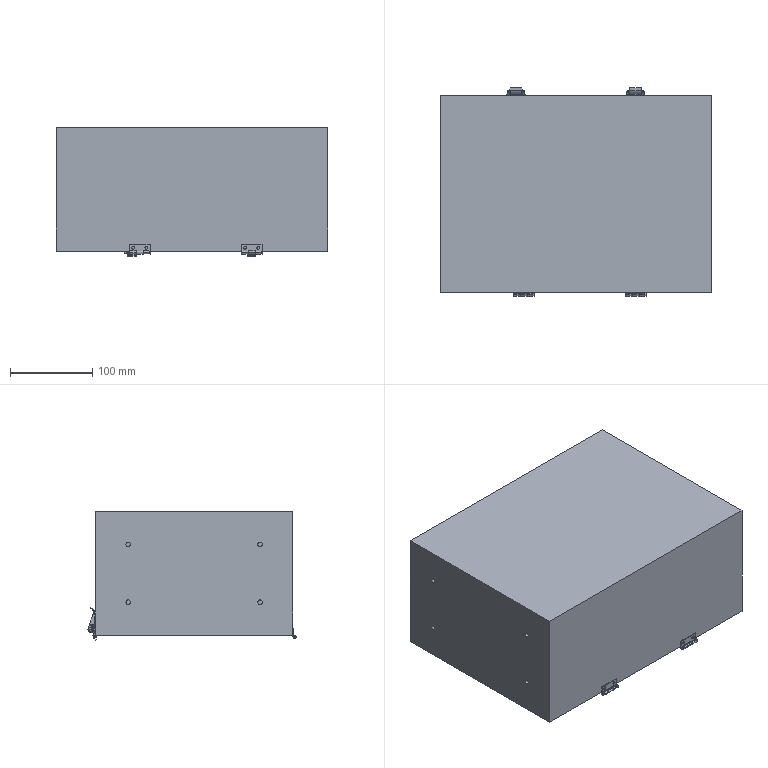Part | SolidWorks | 15 solids | 356 faces | box 330 x 252.816 x 156.5 mm | volume 11874389 mm3 | plane 158 | cylinder 150 | cone 24 | torus 24 | commonest cylinder face diameters 2 x38 3 x26 3.8 x18 3.4 x16 6 x12 5.5 x8